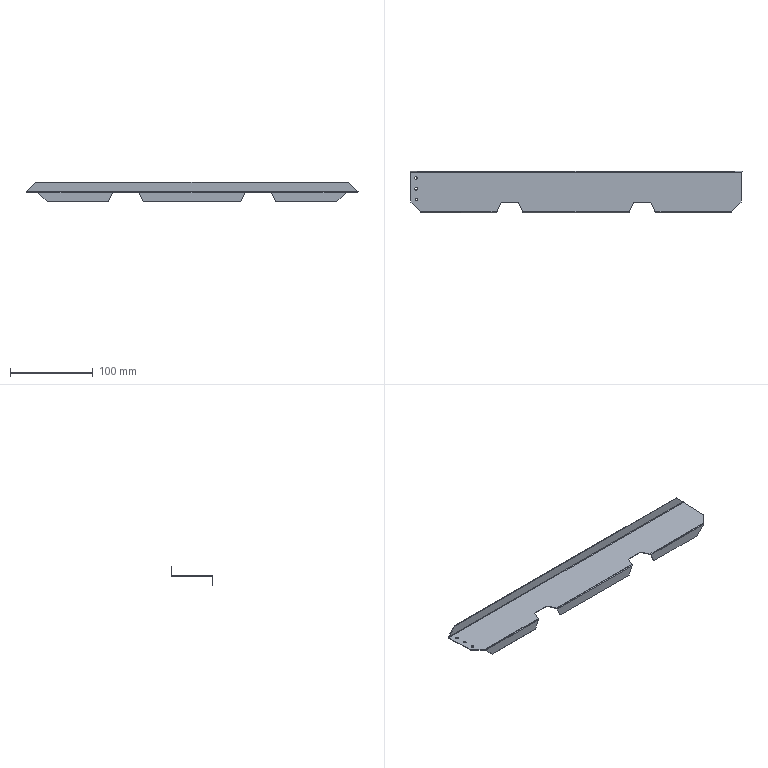Part | SolidWorks | features BaseBody 1 | 1 solid | 56 faces | box 401 x 50 x 24.144 mm | volume 13474 mm3 | plane 32 | cylinder 14 | spline 10 | commonest cylinder face diameters 3.2 x6 1 x4 2 x4